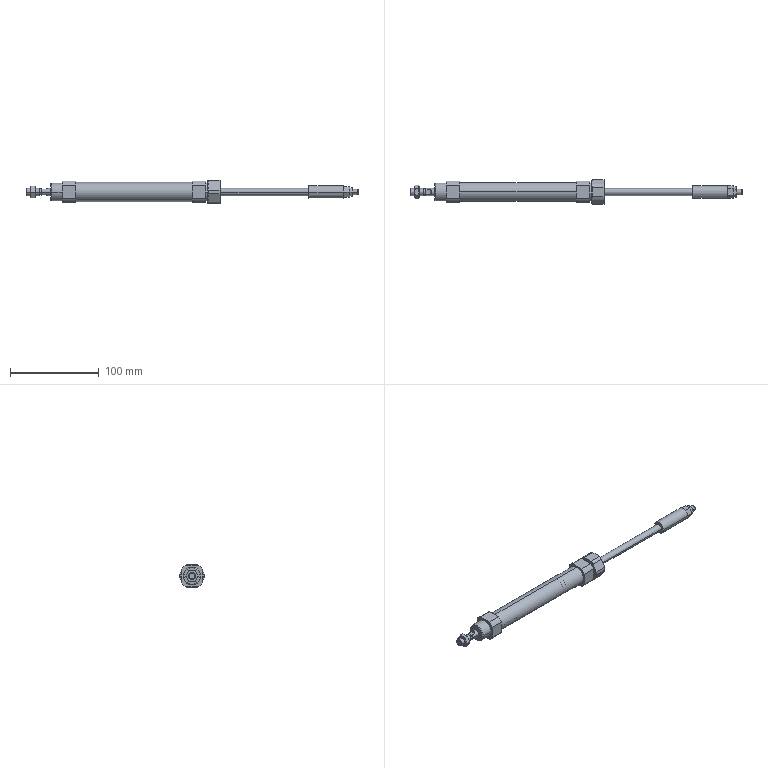Part | 4 solids | 148 faces | box 375 x 28 x 26 mm | volume 63610 mm3 | plane 62 | cylinder 50 | cone 36 | commonest cylinder face diameters 28 x14 8 x12 20 x8 8.566 x4 4.917 x2 6 x2